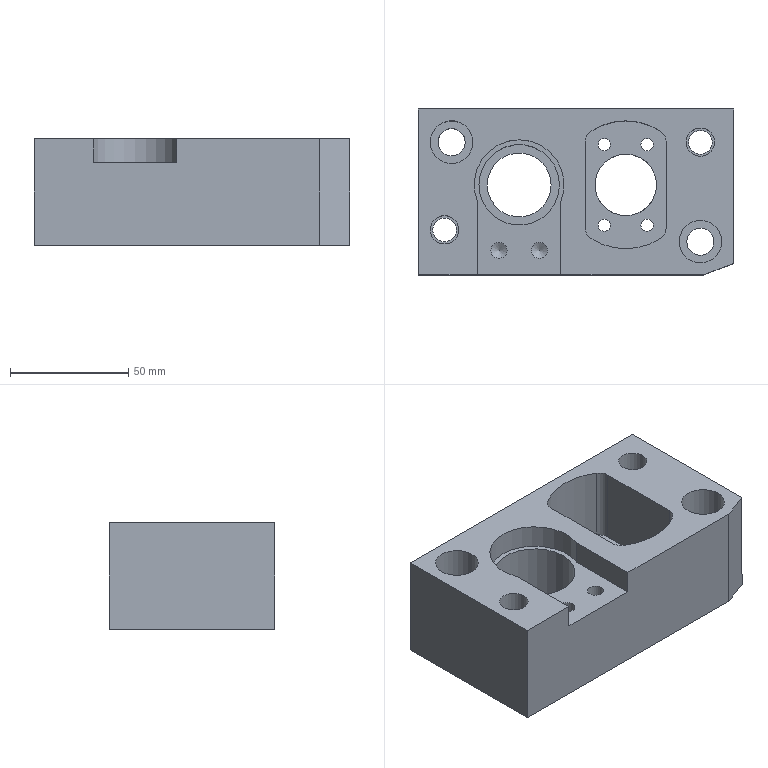Part | NX | features 26 2 | 1 solid | 44 faces | box 133 x 70 x 45 mm | volume 280682 mm3 | cylinder 24 | plane 18 | cone 2 | commonest cylinder face diameters 5.2 x4 10 x4 6.8 x2 10.001 x2 11.5 x2 12 x2
STEP:
#1=CARTESIAN_POINT('',(3287.,18.439,-68.));
#2=VERTEX_POINT('',#1);
#3=CARTESIAN_POINT('',(3287.,-18.439,-68.));
#4=VERTEX_POINT('',#3);
#5=CARTESIAN_POINT('',(3287.,211.,-68.));
#6=DIRECTION('',(0.,-1.,0.));
#7=VECTOR('',#6,1000.);
#8=LINE('',#5,#7);
#9=EDGE_CURVE('',#2,#4,#8,.T.);
#10=ORIENTED_EDGE('',*,*,#9,.F.);
#11=CARTESIAN_POINT('',(3289.273,22.63,-68.));
#12=VERTEX_POINT('',#11);
#13=CARTESIAN_POINT('',(3292.,18.439,-68.));
#14=DIRECTION('',(0.,0.,1.));
#15=DIRECTION('',(1.,0.,0.));
#16=AXIS2_PLACEMENT_3D('',#13,#14,#15);
#17=CIRCLE('',#16,5.);
#18=EDGE_CURVE('',#12,#2,#17,.T.);
#19=ORIENTED_EDGE('',*,*,#18,.F.);
#20=CARTESIAN_POINT('',(3318.727,22.63,-68.));
#21=VERTEX_POINT('',#20);
#22=CARTESIAN_POINT('',(3304.,0.,-68.));
#23=DIRECTION('',(0.,0.,1.));
#24=DIRECTION('',(1.,0.,0.));
#25=AXIS2_PLACEMENT_3D('',#22,#23,#24);
#26=CIRCLE('',#25,27.);
#27=EDGE_CURVE('',#21,#12,#26,.T.);
#28=ORIENTED_EDGE('',*,*,#27,.F.);
#29=CARTESIAN_POINT('',(3321.,18.439,-68.));
#30=VERTEX_POINT('',#29);
#31=CARTESIAN_POINT('',(3316.,18.439,-68.));
#32=DIRECTION('',(0.,0.,1.));
#33=DIRECTION('',(1.,0.,0.));
#34=AXIS2_PLACEMENT_3D('',#31,#32,#33);
#35=CIRCLE('',#34,5.);
#36=EDGE_CURVE('',#30,#21,#35,.T.);
#37=ORIENTED_EDGE('',*,*,#36,.F.);
#38=CARTESIAN_POINT('',(3321.,-18.439,-68.));
#39=VERTEX_POINT('',#38);
#40=CARTESIAN_POINT('',(3321.,211.,-68.));
#41=DIRECTION('',(0.,1.,0.));
#42=VECTOR('',#41,1000.);
#43=LINE('',#40,#42);
#44=EDGE_CURVE('',#39,#30,#43,.T.);
#45=ORIENTED_EDGE('',*,*,#44,.F.);
#46=CARTESIAN_POINT('',(3318.727,-22.63,-68.));
#47=VERTEX_POINT('',#46);
#48=CARTESIAN_POINT('',(3316.,-18.439,-68.));
#49=DIRECTION('',(0.,0.,1.));
#50=DIRECTION('',(1.,0.,0.));
#51=AXIS2_PLACEMENT_3D('',#48,#49,#50);
#52=CIRCLE('',#51,5.);
#53=EDGE_CURVE('',#47,#39,#52,.T.);
#54=ORIENTED_EDGE('',*,*,#53,.F.);
#55=CARTESIAN_POINT('',(3289.273,-22.63,-68.));
#56=VERTEX_POINT('',#55);
#57=CARTESIAN_POINT('',(3304.,0.,-68.));
#58=DIRECTION('',(0.,0.,1.));
#59=DIRECTION('',(1.,0.,0.));
#60=AXIS2_PLACEMENT_3D('',#57,#58,#59);
#61=CIRCLE('',#60,27.);
#62=EDGE_CURVE('',#56,#47,#61,.T.);
#63=ORIENTED_EDGE('',*,*,#62,.F.);
#64=CARTESIAN_POINT('',(3292.,-18.439,-68.));
#65=DIRECTION('',(0.,0.,1.));
#66=DIRECTION('',(1.,0.,0.));
#67=AXIS2_PLACEMENT_3D('',#64,#65,#66);
#68=CIRCLE('',#67,5.);
#69=EDGE_CURVE('',#4,#56,#68,.T.);
#70=ORIENTED_EDGE('',*,*,#69,.F.);
#71=EDGE_LOOP('',(#10,#19,#28,#37,#45,#54,#63,#70));
#72=FACE_BOUND('',#71,.T.);
#73=CARTESIAN_POINT('',(3326.5,-24.,-68.));
#74=VERTEX_POINT('',#73);
#75=CARTESIAN_POINT('',(3335.5,-24.,-68.));
#76=DIRECTION('',(0.,0.,1.));
#77=DIRECTION('',(-1.,0.,0.));
#78=AXIS2_PLACEMENT_3D('',#75,#76,#77);
#79=CIRCLE('',#78,9.);
#80=EDGE_CURVE('',#74,#74,#79,.T.);
#81=ORIENTED_EDGE('',*,*,#80,.F.);
#82=EDGE_LOOP('',(#81));
#83=FACE_BOUND('',#82,.T.);
#84=CARTESIAN_POINT('',(3221.5,18.,-68.));
#85=VERTEX_POINT('',#84);
#86=CARTESIAN_POINT('',(3230.5,18.,-68.));
#87=DIRECTION('',(0.,0.,1.));
#88=DIRECTION('',(-1.,0.,0.));
#89=AXIS2_PLACEMENT_3D('',#86,#87,#88);
#90=CIRCLE('',#89,9.);
#91=EDGE_CURVE('',#85,#85,#90,.T.);
#92=ORIENTED_EDGE('',*,*,#91,.F.);
#93=EDGE_LOOP('',(#92));
#94=FACE_BOUND('',#93,.T.);
#95=CARTESIAN_POINT('',(3233.5,-19.,-68.));
#96=VERTEX_POINT('',#95);
#97=CARTESIAN_POINT('',(3227.5,-19.,-68.));
#98=DIRECTION('',(0.,0.,-1.));
#99=DIRECTION('',(1.,0.,0.));
#100=AXIS2_PLACEMENT_3D('',#97,#98,#99);
#101=CIRCLE('',#100,6.);
#102=EDGE_CURVE('',#96,#96,#101,.T.);
#103=ORIENTED_EDGE('',*,*,#102,.T.);
#104=EDGE_LOOP('',(#103));
#105=FACE_BOUND('',#104,.T.);
#106=CARTESIAN_POINT('',(3341.5,18.,-68.));
#107=VERTEX_POINT('',#106);
#108=CARTESIAN_POINT('',(3335.5,18.,-68.));
#109=DIRECTION('',(0.,0.,-1.));
#110=DIRECTION('',(1.,0.,0.));
#111=AXIS2_PLACEMENT_3D('',#108,#109,#110);
#112=CIRCLE('',#111,6.);
#113=EDGE_CURVE('',#107,#107,#112,.T.);
#114=ORIENTED_EDGE('',*,*,#113,.T.);
#115=EDGE_LOOP('',(#114));
#116=FACE_BOUND('',#115,.T.);
#117=CARTESIAN_POINT('',(3349.5,-33.209,-68.));
#118=VERTEX_POINT('',#117);
#119=CARTESIAN_POINT('',(3336.859,-38.,-68.));
#120=VERTEX_POINT('',#119);
#121=CARTESIAN_POINT('',(4367.889,352.74,-68.));
#122=DIRECTION('',(-0.9351,-0.3544,0.));
#123=VECTOR('',#122,1000.);
#124=LINE('',#121,#123);
#125=EDGE_CURVE('',#118,#120,#124,.T.);
#126=ORIENTED_EDGE('',*,*,#125,.F.);
#127=CARTESIAN_POINT('',(3349.5,32.,-68.));
#128=VERTEX_POINT('',#127);
#129=CARTESIAN_POINT('',(3349.5,0.,-68.));
#130=DIRECTION('',(0.,1.,0.));
#131=VECTOR('',#130,1000.);
#132=LINE('',#129,#131);
#133=EDGE_CURVE('',#118,#128,#132,.T.);
#134=ORIENTED_EDGE('',*,*,#133,.T.);
#135=CARTESIAN_POINT('',(3216.5,32.,-68.));
#136=VERTEX_POINT('',#135);
#137=CARTESIAN_POINT('',(3259.,32.,-68.));
#138=DIRECTION('',(-1.,0.,0.));
#139=VECTOR('',#138,1000.);
#140=LINE('',#137,#139);
#141=EDGE_CURVE('',#128,#136,#140,.T.);
#142=ORIENTED_EDGE('',*,*,#141,.T.);
#143=CARTESIAN_POINT('',(3216.5,-38.,-68.));
#144=VERTEX_POINT('',#143);
#145=CARTESIAN_POINT('',(3216.5,0.,-68.));
#146=DIRECTION('',(0.,-1.,0.));
#147=VECTOR('',#146,1000.);
#148=LINE('',#145,#147);
#149=EDGE_CURVE('',#136,#144,#148,.T.);
#150=ORIENTED_EDGE('',*,*,#149,.T.);
#151=CARTESIAN_POINT('',(3241.4,-38.,-68.));
#152=VERTEX_POINT('',#151);
#153=CARTESIAN_POINT('',(3259.,-38.,-68.));
#154=DIRECTION('',(1.,0.,0.));
#155=VECTOR('',#154,1000.);
#156=LINE('',#153,#155);
#157=EDGE_CURVE('',#144,#152,#156,.T.);
#158=ORIENTED_EDGE('',*,*,#157,.T.);
#159=CARTESIAN_POINT('',(3241.4,-7.158,-68.));
#160=VERTEX_POINT('',#159);
#161=CARTESIAN_POINT('',(3241.4,206.,-68.));
#162=DIRECTION('',(0.,-1.,0.));
#163=VECTOR('',#162,1000.);
#164=LINE('',#161,#163);
#165=EDGE_CURVE('',#160,#152,#164,.T.);
#166=ORIENTED_EDGE('',*,*,#165,.F.);
#167=CARTESIAN_POINT('',(3276.6,-7.158,-68.));
#168=VERTEX_POINT('',#167);
#169=CARTESIAN_POINT('',(3259.,0.,-68.));
#170=DIRECTION('',(0.,0.,1.));
#171=DIRECTION('',(-1.,0.,0.));
#172=AXIS2_PLACEMENT_3D('',#169,#170,#171);
#173=CIRCLE('',#172,19.);
#174=EDGE_CURVE('',#168,#160,#173,.T.);
#175=ORIENTED_EDGE('',*,*,#174,.F.);
#176=CARTESIAN_POINT('',(3276.6,-38.,-68.));
#177=VERTEX_POINT('',#176);
#178=CARTESIAN_POINT('',(3276.6,206.,-68.));
#179=DIRECTION('',(0.,1.,0.));
#180=VECTOR('',#179,1000.);
#181=LINE('',#178,#180);
#182=EDGE_CURVE('',#177,#168,#181,.T.);
#183=ORIENTED_EDGE('',*,*,#182,.F.);
#184=CARTESIAN_POINT('',(3259.,-38.,-68.));
#185=DIRECTION('',(1.,0.,0.));
#186=VECTOR('',#185,1000.);
#187=LINE('',#184,#186);
#188=EDGE_CURVE('',#177,#120,#187,.T.);
#189=ORIENTED_EDGE('',*,*,#188,.T.);
#190=EDGE_LOOP('',(#126,#134,#142,#150,#158,#166,#175,#183,#189));
#191=FACE_BOUND('',#190,.T.);
#192=CARTESIAN_POINT('',(4423.5,206.,-68.));
#193=DIRECTION('',(0.,0.,-1.));
#194=DIRECTION('',(1.,0.,0.));
#195=AXIS2_PLACEMENT_3D('',#192,#193,#194);
#196=PLANE('',#195);
#197=ADVANCED_FACE('',(#72,#83,#94,#105,#116,#191),#196,.F.);
#198=ORIENTED_EDGE('',*,*,#133,.F.);
#199=CARTESIAN_POINT('',(3349.5,-33.209,-113.));
#200=VERTEX_POINT('',#199);
#201=CARTESIAN_POINT('',(3349.5,-33.209,-123.5));
#202=DIRECTION('',(0.,0.,-1.));
#203=VECTOR('',#202,1000.);
#204=LINE('',#201,#203);
#205=EDGE_CURVE('',#118,#200,#204,.T.);
#206=ORIENTED_EDGE('',*,*,#205,.T.);
#207=CARTESIAN_POINT('',(3349.5,32.,-113.));
#208=VERTEX_POINT('',#207);
#209=CARTESIAN_POINT('',(3349.5,0.,-113.));
#210=DIRECTION('',(0.,-1.,0.));
#211=VECTOR('',#210,1000.);
#212=LINE('',#209,#211);
#213=EDGE_CURVE('',#208,#200,#212,.T.);
#214=ORIENTED_EDGE('',*,*,#213,.F.);
#215=CARTESIAN_POINT('',(3349.5,32.,-123.5));
#216=DIRECTION('',(0.,0.,1.));
#217=VECTOR('',#216,1000.);
#218=LINE('',#215,#217);
#219=EDGE_CURVE('',#208,#128,#218,.T.);
#220=ORIENTED_EDGE('',*,*,#219,.T.);
#221=EDGE_LOOP('',(#198,#206,#214,#220));
#222=FACE_BOUND('',#221,.T.);
#223=CARTESIAN_POINT('',(3349.5,0.,-123.5));
#224=DIRECTION('',(1.,0.,0.));
#225=DIRECTION('',(0.,0.,1.));
#226=AXIS2_PLACEMENT_3D('',#223,#224,#225);
#227=PLANE('',#226);
#228=ADVANCED_FACE('',(#222),#227,.T.);
#229=CARTESIAN_POINT('',(3336.859,-38.,-113.));
#230=VERTEX_POINT('',#229);
#231=CARTESIAN_POINT('',(3216.5,-38.,-113.));
#232=VERTEX_POINT('',#231);
#233=CARTESIAN_POINT('',(3259.,-38.,-113.));
#234=DIRECTION('',(-1.,0.,0.));
#235=VECTOR('',#234,1000.);
#236=LINE('',#233,#235);
#237=EDGE_CURVE('',#230,#232,#236,.T.);
#238=ORIENTED_EDGE('',*,*,#237,.F.);
#239=CARTESIAN_POINT('',(3336.859,-38.,-123.5));
#240=DIRECTION('',(0.,0.,1.));
#241=VECTOR('',#240,1000.);
#242=LINE('',#239,#241);
#243=EDGE_CURVE('',#230,#120,#242,.T.);
#244=ORIENTED_EDGE('',*,*,#243,.T.);
#245=ORIENTED_EDGE('',*,*,#188,.F.);
#246=CARTESIAN_POINT('',(3276.6,-38.,-78.));
#247=VERTEX_POINT('',#246);
#248=CARTESIAN_POINT('',(3276.6,-38.,-123.5));
#249=DIRECTION('',(0.,0.,-1.));
#250=VECTOR('',#249,1000.);
#251=LINE('',#248,#250);
#252=EDGE_CURVE('',#177,#247,#251,.T.);
#253=ORIENTED_EDGE('',*,*,#252,.T.);
#254=CARTESIAN_POINT('',(3241.4,-38.,-78.));
#255=VERTEX_POINT('',#254);
#256=CARTESIAN_POINT('',(3259.,-38.,-78.));
#257=DIRECTION('',(-1.,0.,0.));
#258=VECTOR('',#257,1000.);
#259=LINE('',#256,#258);
#260=EDGE_CURVE('',#247,#255,#259,.T.);
#261=ORIENTED_EDGE('',*,*,#260,.T.);
#262=CARTESIAN_POINT('',(3241.4,-38.,-58.));
#263=DIRECTION('',(0.,0.,-1.));
#264=VECTOR('',#263,1000.);
#265=LINE('',#262,#264);
#266=EDGE_CURVE('',#152,#255,#265,.T.);
#267=ORIENTED_EDGE('',*,*,#266,.F.);
#268=ORIENTED_EDGE('',*,*,#157,.F.);
#269=CARTESIAN_POINT('',(3216.5,-38.,-123.5));
#270=DIRECTION('',(0.,0.,1.));
#271=VECTOR('',#270,1000.);
#272=LINE('',#269,#271);
#273=EDGE_CURVE('',#232,#144,#272,.T.);
#274=ORIENTED_EDGE('',*,*,#273,.F.);
#275=EDGE_LOOP('',(#238,#244,#245,#253,#261,#267,#268,#274));
#276=FACE_BOUND('',#275,.T.);
#277=CARTESIAN_POINT('',(3259.,-38.,-123.5));
#278=DIRECTION('',(0.,-1.,0.));
#279=DIRECTION('',(0.,0.,-1.));
#280=AXIS2_PLACEMENT_3D('',#277,#278,#279);
#281=PLANE('',#280);
#282=ADVANCED_FACE('',(#276),#281,.T.);
#283=CARTESIAN_POINT('',(3292.4,17.,-113.));
#284=VERTEX_POINT('',#283);
#285=CARTESIAN_POINT('',(3295.,17.,-113.));
#286=DIRECTION('',(0.,0.,-1.));
#287=DIRECTION('',(-1.,0.,0.));
#288=AXIS2_PLACEMENT_3D('',#285,#286,#287);
#289=CIRCLE('',#288,2.6);
#290=EDGE_CURVE('',#284,#284,#289,.T.);
#291=ORIENTED_EDGE('',*,*,#290,.F.);
#292=EDGE_LOOP('',(#291));
#293=FACE_BOUND('',#292,.T.);
#294=CARTESIAN_POINT('',(3292.4,-17.,-113.));
#295=VERTEX_POINT('',#294);
#296=CARTESIAN_POINT('',(3295.,-17.,-113.));
#297=DIRECTION('',(0.,0.,-1.));
#298=DIRECTION('',(-1.,0.,0.));
#299=AXIS2_PLACEMENT_3D('',#296,#297,#298);
#300=CIRCLE('',#299,2.6);
#301=EDGE_CURVE('',#295,#295,#300,.T.);
#302=ORIENTED_EDGE('',*,*,#301,.F.);
#303=EDGE_LOOP('',(#302));
#304=FACE_BOUND('',#303,.T.);
#305=CARTESIAN_POINT('',(3310.4,17.,-113.));
#306=VERTEX_POINT('',#305);
#307=CARTESIAN_POINT('',(3313.,17.,-113.));
#308=DIRECTION('',(0.,0.,-1.));
#309=DIRECTION('',(-1.,0.,0.));
#310=AXIS2_PLACEMENT_3D('',#307,#308,#309);
#311=CIRCLE('',#310,2.6);
#312=EDGE_CURVE('',#306,#306,#311,.T.);
#313=ORIENTED_EDGE('',*,*,#312,.F.);
#314=EDGE_LOOP('',(#313));
#315=FACE_BOUND('',#314,.T.);
#316=CARTESIAN_POINT('',(3310.4,-17.,-113.));
#317=VERTEX_POINT('',#316);
#318=CARTESIAN_POINT('',(3313.,-17.,-113.));
#319=DIRECTION('',(0.,0.,-1.));
#320=DIRECTION('',(-1.,0.,0.));
#321=AXIS2_PLACEMENT_3D('',#318,#319,#320);
#322=CIRCLE('',#321,2.6);
#323=EDGE_CURVE('',#317,#317,#322,.T.);
#324=ORIENTED_EDGE('',*,*,#323,.F.);
#325=EDGE_LOOP('',(#324));
#326=FACE_BOUND('',#325,.T.);
#327=CARTESIAN_POINT('',(3222.499,-19.,-113.));
#328=VERTEX_POINT('',#327);
#329=CARTESIAN_POINT('',(3227.5,-19.,-113.));
#330=DIRECTION('',(0.,0.,-1.));
#331=DIRECTION('',(-1.,0.,0.));
#332=AXIS2_PLACEMENT_3D('',#329,#330,#331);
#333=CIRCLE('',#332,5.);
#334=EDGE_CURVE('',#328,#328,#333,.T.);
#335=ORIENTED_EDGE('',*,*,#334,.F.);
#336=EDGE_LOOP('',(#335));
#337=FACE_BOUND('',#336,.T.);
#338=CARTESIAN_POINT('',(3224.75,18.,-113.));
#339=VERTEX_POINT('',#338);
#340=CARTESIAN_POINT('',(3230.5,18.,-113.));
#341=DIRECTION('',(0.,0.,-1.));
#342=DIRECTION('',(-1.,0.,0.));
#343=AXIS2_PLACEMENT_3D('',#340,#341,#342);
#344=CIRCLE('',#343,5.75);
#345=EDGE_CURVE('',#339,#339,#344,.T.);
#346=ORIENTED_EDGE('',*,*,#345,.F.);
#347=EDGE_LOOP('',(#346));
#348=FACE_BOUND('',#347,.T.);
#349=CARTESIAN_POINT('',(3245.5,0.,-113.));
#350=VERTEX_POINT('',#349);
#351=CARTESIAN_POINT('',(3259.,0.,-113.));
#352=DIRECTION('',(0.,0.,-1.));
#353=DIRECTION('',(-1.,0.,0.));
#354=AXIS2_PLACEMENT_3D('',#351,#352,#353);
#355=CIRCLE('',#354,13.5);
#356=EDGE_CURVE('',#350,#350,#355,.T.);
#357=ORIENTED_EDGE('',*,*,#356,.F.);
#358=EDGE_LOOP('',(#357));
#359=FACE_BOUND('',#358,.T.);
#360=CARTESIAN_POINT('',(3329.75,-24.,-113.));
#361=VERTEX_POINT('',#360);
#362=CARTESIAN_POINT('',(3335.5,-24.,-113.));
#363=DIRECTION('',(0.,0.,-1.));
#364=DIRECTION('',(-1.,0.,0.));
#365=AXIS2_PLACEMENT_3D('',#362,#363,#364);
#366=CIRCLE('',#365,5.75);
#367=EDGE_CURVE('',#361,#361,#366,.T.);
#368=ORIENTED_EDGE('',*,*,#367,.F.);
#369=EDGE_LOOP('',(#368));
#370=FACE_BOUND('',#369,.T.);
#371=CARTESIAN_POINT('',(3330.499,18.,-113.));
#372=VERTEX_POINT('',#371);
#373=CARTESIAN_POINT('',(3335.5,18.,-113.));
#374=DIRECTION('',(0.,0.,-1.));
#375=DIRECTION('',(-1.,0.,0.));
#376=AXIS2_PLACEMENT_3D('',#373,#374,#375);
#377=CIRCLE('',#376,5.);
#378=EDGE_CURVE('',#372,#372,#377,.T.);
#379=ORIENTED_EDGE('',*,*,#378,.F.);
#380=EDGE_LOOP('',(#379));
#381=FACE_BOUND('',#380,.T.);
#382=CARTESIAN_POINT('',(3317.,0.,-113.));
#383=VERTEX_POINT('',#382);
#384=CARTESIAN_POINT('',(3304.,0.,-113.));
#385=DIRECTION('',(0.,0.,1.));
#386=DIRECTION('',(1.,0.,0.));
#387=AXIS2_PLACEMENT_3D('',#384,#385,#386);
#388=CIRCLE('',#387,13.);
#389=EDGE_CURVE('',#383,#383,#388,.T.);
#390=ORIENTED_EDGE('',*,*,#389,.T.);
#391=EDGE_LOOP('',(#390));
#392=FACE_BOUND('',#391,.T.);
#393=ORIENTED_EDGE('',*,*,#213,.T.);
#394=CARTESIAN_POINT('',(4355.903,348.197,-113.));
#395=DIRECTION('',(-0.9351,-0.3544,0.));
#396=VECTOR('',#395,1000.);
#397=LINE('',#394,#396);
#398=EDGE_CURVE('',#200,#230,#397,.T.);
#399=ORIENTED_EDGE('',*,*,#398,.T.);
#400=ORIENTED_EDGE('',*,*,#237,.T.);
#401=CARTESIAN_POINT('',(3216.5,32.,-113.));
#402=VERTEX_POINT('',#401);
#403=CARTESIAN_POINT('',(3216.5,0.,-113.));
#404=DIRECTION('',(0.,1.,0.));
#405=VECTOR('',#404,1000.);
#406=LINE('',#403,#405);
#407=EDGE_CURVE('',#232,#402,#406,.T.);
#408=ORIENTED_EDGE('',*,*,#407,.T.);
#409=CARTESIAN_POINT('',(3259.,32.,-113.));
#410=DIRECTION('',(1.,0.,0.));
#411=VECTOR('',#410,1000.);
#412=LINE('',#409,#411);
#413=EDGE_CURVE('',#402,#208,#412,.T.);
#414=ORIENTED_EDGE('',*,*,#413,.T.);
#415=EDGE_LOOP('',(#393,#399,#400,#408,#414));
#416=FACE_BOUND('',#415,.T.);
#417=CARTESIAN_POINT('',(4489.,-3.,-113.));
#418=DIRECTION('',(0.,0.,-1.));
#419=DIRECTION('',(-1.,0.,0.));
#420=AXIS2_PLACEMENT_3D('',#417,#418,#419);
#421=PLANE('',#420);
#422=ADVANCED_FACE('',(#293,#304,#315,#326,#337,#348,#359,#370,#381,#392,#416),#421,.T.);
#423=CARTESIAN_POINT('',(3276.,0.,-108.));
#424=VERTEX_POINT('',#423);
#425=CARTESIAN_POINT('',(3259.,0.,-108.));
#426=DIRECTION('',(0.,0.,1.));
#427=DIRECTION('',(1.,0.,0.));
#428=AXIS2_PLACEMENT_3D('',#425,#426,#427);
#429=CIRCLE('',#428,17.);
#430=EDGE_CURVE('',#424,#424,#429,.T.);
#431=ORIENTED_EDGE('',*,*,#430,.F.);
#432=EDGE_LOOP('',(#431));
#433=FACE_BOUND('',#432,.T.);
#434=CARTESIAN_POINT('',(3276.,0.,-78.));
#435=VERTEX_POINT('',#434);
#436=CARTESIAN_POINT('',(3259.,0.,-78.));
#437=DIRECTION('',(0.,0.,-1.));
#438=DIRECTION('',(1.,0.,0.));
#439=AXIS2_PLACEMENT_3D('',#436,#437,#438);
#440=CIRCLE('',#439,17.);
#441=EDGE_CURVE('',#435,#435,#440,.T.);
#442=ORIENTED_EDGE('',*,*,#441,.F.);
#443=EDGE_LOOP('',(#442));
#444=FACE_BOUND('',#443,.T.);
#445=CARTESIAN_POINT('',(3259.,0.,512.));
#446=DIRECTION('',(0.,0.,-1.));
#447=DIRECTION('',(1.,0.,0.));
#448=AXIS2_PLACEMENT_3D('',#445,#446,#447);
#449=CYLINDRICAL_SURFACE('',#448,17.);
#450=ADVANCED_FACE('',(#433,#444),#449,.F.);
#451=ORIENTED_EDGE('',*,*,#273,.T.);
#452=ORIENTED_EDGE('',*,*,#149,.F.);
#453=CARTESIAN_POINT('',(3216.5,32.,-123.5));
#454=DIRECTION('',(0.,0.,1.));
#455=VECTOR('',#454,1000.);
#456=LINE('',#453,#455);
#457=EDGE_CURVE('',#402,#136,#456,.T.);
#458=ORIENTED_EDGE('',*,*,#457,.F.);
#459=ORIENTED_EDGE('',*,*,#407,.F.);
#460=EDGE_LOOP('',(#451,#452,#458,#459));
#461=FACE_BOUND('',#460,.T.);
#462=CARTESIAN_POINT('',(3216.5,0.,-123.5));
#463=DIRECTION('',(-1.,0.,0.));
#464=DIRECTION('',(0.,0.,-1.));
#465=AXIS2_PLACEMENT_3D('',#462,#463,#464);
#466=PLANE('',#465);
#467=ADVANCED_FACE('',(#461),#466,.T.);
#468=ORIENTED_EDGE('',*,*,#457,.T.);
#469=ORIENTED_EDGE('',*,*,#141,.F.);
#470=ORIENTED_EDGE('',*,*,#219,.F.);
#471=ORIENTED_EDGE('',*,*,#413,.F.);
#472=EDGE_LOOP('',(#468,#469,#470,#471));
#473=FACE_BOUND('',#472,.T.);
#474=CARTESIAN_POINT('',(3259.,32.,-123.5));
#475=DIRECTION('',(0.,1.,0.));
#476=DIRECTION('',(0.,0.,1.));
#477=AXIS2_PLACEMENT_3D('',#474,#475,#476);
#478=PLANE('',#477);
#479=ADVANCED_FACE('',(#473),#478,.T.);
#480=CARTESIAN_POINT('',(3222.499,-19.,-88.5));
#481=VERTEX_POINT('',#480);
#482=CARTESIAN_POINT('',(3227.5,-19.,-88.5));
#483=DIRECTION('',(0.,0.,1.));
#484=DIRECTION('',(-1.,0.,0.));
#485=AXIS2_PLACEMENT_3D('',#482,#483,#484);
#486=CIRCLE('',#485,5.);
#487=EDGE_CURVE('',#481,#481,#486,.T.);
#488=ORIENTED_EDGE('',*,*,#487,.T.);
#489=EDGE_LOOP('',(#488));
#490=FACE_BOUND('',#489,.T.);
#491=ORIENTED_EDGE('',*,*,#334,.T.);
#492=EDGE_LOOP('',(#491));
#493=FACE_BOUND('',#492,.T.);
#494=CARTESIAN_POINT('',(3227.5,-19.,541.5));
#495=DIRECTION('',(0.,0.,-1.));
#496=DIRECTION('',(1.,0.,0.));
#497=AXIS2_PLACEMENT_3D('',#494,#495,#496);
#498=CYLINDRICAL_SURFACE('',#497,5.);
#499=ADVANCED_FACE('',(#490,#493),#498,.F.);
#500=CARTESIAN_POINT('',(3330.499,18.,-88.5));
#501=VERTEX_POINT('',#500);
#502=CARTESIAN_POINT('',(3335.5,18.,-88.5));
#503=DIRECTION('',(0.,0.,1.));
#504=DIRECTION('',(-1.,0.,0.));
#505=AXIS2_PLACEMENT_3D('',#502,#503,#504);
#506=CIRCLE('',#505,5.);
#507=EDGE_CURVE('',#501,#501,#506,.T.);
#508=ORIENTED_EDGE('',*,*,#507,.T.);
#509=EDGE_LOOP('',(#508));
#510=FACE_BOUND('',#509,.T.);
#511=ORIENTED_EDGE('',*,*,#378,.T.);
#512=EDGE_LOOP('',(#511));
#513=FACE_BOUND('',#512,.T.);
#514=CARTESIAN_POINT('',(3335.5,18.,541.5));
#515=DIRECTION('',(0.,0.,-1.));
#516=DIRECTION('',(1.,0.,0.));
#517=AXIS2_PLACEMENT_3D('',#514,#515,#516);
#518=CYLINDRICAL_SURFACE('',#517,5.);
#519=ADVANCED_FACE('',(#510,#513),#518,.F.);
#520=CARTESIAN_POINT('',(3224.75,18.,-88.5));
#521=VERTEX_POINT('',#520);
#522=CARTESIAN_POINT('',(3230.5,18.,-88.5));
#523=DIRECTION('',(0.,0.,1.));
#524=DIRECTION('',(-1.,0.,0.));
#525=AXIS2_PLACEMENT_3D('',#522,#523,#524);
#526=CIRCLE('',#525,5.75);
#527=EDGE_CURVE('',#521,#521,#526,.T.);
#528=ORIENTED_EDGE('',*,*,#527,.T.);
#529=EDGE_LOOP('',(#528));
#530=FACE_BOUND('',#529,.T.);
#531=ORIENTED_EDGE('',*,*,#345,.T.);
#532=EDGE_LOOP('',(#531));
#533=FACE_BOUND('',#532,.T.);
#534=CARTESIAN_POINT('',(3230.5,18.,-66.5));
#535=DIRECTION('',(0.,0.,-1.));
#536=DIRECTION('',(-1.,0.,0.));
#537=AXIS2_PLACEMENT_3D('',#534,#535,#536);
#538=CYLINDRICAL_SURFACE('',#537,5.75);
#539=ADVANCED_FACE('',(#530,#533),#538,.F.);
#540=CARTESIAN_POINT('',(3329.75,-24.,-88.5));
#541=VERTEX_POINT('',#540);
#542=CARTESIAN_POINT('',(3335.5,-24.,-88.5));
#543=DIRECTION('',(0.,0.,1.));
#544=DIRECTION('',(-1.,0.,0.));
#545=AXIS2_PLACEMENT_3D('',#542,#543,#544);
#546=CIRCLE('',#545,5.75);
#547=EDGE_CURVE('',#541,#541,#546,.T.);
#548=ORIENTED_EDGE('',*,*,#547,.T.);
#549=EDGE_LOOP('',(#548));
#550=FACE_BOUND('',#549,.T.);
#551=ORIENTED_EDGE('',*,*,#367,.T.);
#552=EDGE_LOOP('',(#551));
#553=FACE_BOUND('',#552,.T.);
#554=CARTESIAN_POINT('',(3335.5,-24.,-66.5));
#555=DIRECTION('',(0.,0.,-1.));
#556=DIRECTION('',(-1.,0.,0.));
#557=AXIS2_PLACEMENT_3D('',#554,#555,#556);
#558=CYLINDRICAL_SURFACE('',#557,5.75);
#559=ADVANCED_FACE('',(#550,#553),#558,.F.);
#560=CARTESIAN_POINT('',(3272.5,0.,-108.));
#561=VERTEX_POINT('',#560);
#562=CARTESIAN_POINT('',(3259.,0.,-108.));
#563=DIRECTION('',(0.,0.,1.));
#564=DIRECTION('',(1.,0.,0.));
#565=AXIS2_PLACEMENT_3D('',#562,#563,#564);
#566=CIRCLE('',#565,13.5);
#567=EDGE_CURVE('',#561,#561,#566,.T.);
#568=ORIENTED_EDGE('',*,*,#567,.T.);
#569=EDGE_LOOP('',(#568));
#570=FACE_BOUND('',#569,.T.);
#571=ORIENTED_EDGE('',*,*,#356,.T.);
#572=EDGE_LOOP('',(#571));
#573=FACE_BOUND('',#572,.T.);
#574=CARTESIAN_POINT('',(3259.,0.,542.));
#575=DIRECTION('',(0.,0.,-1.));
#576=DIRECTION('',(1.,0.,0.));
#577=AXIS2_PLACEMENT_3D('',#574,#575,#576);
#578=CYLINDRICAL_SURFACE('',#577,13.5);
#579=ADVANCED_FACE('',(#570,#573),#578,.F.);
#580=CARTESIAN_POINT('',(3329.5,18.,-88.5));
#581=VERTEX_POINT('',#580);
#582=CARTESIAN_POINT('',(3335.5,18.,-88.5));
#583=DIRECTION('',(0.,0.,-1.));
#584=DIRECTION('',(-1.,0.,0.));
#585=AXIS2_PLACEMENT_3D('',#582,#583,#584);
#586=CIRCLE('',#585,6.);
#587=EDGE_CURVE('',#581,#581,#586,.T.);
#588=ORIENTED_EDGE('',*,*,#587,.T.);
#589=EDGE_LOOP('',(#588));
#590=FACE_BOUND('',#589,.T.);
#591=ORIENTED_EDGE('',*,*,#113,.F.);
#592=EDGE_LOOP('',(#591));
#593=FACE_BOUND('',#592,.T.);
#594=CARTESIAN_POINT('',(3335.5,18.,541.5));
#595=DIRECTION('',(0.,0.,-1.));
#596=DIRECTION('',(1.,0.,0.));
#597=AXIS2_PLACEMENT_3D('',#594,#595,#596);
#598=CYLINDRICAL_SURFACE('',#597,6.);
#599=ADVANCED_FACE('',(#590,#593),#598,.F.);
#600=CARTESIAN_POINT('',(3221.5,-19.,-88.5));
#601=VERTEX_POINT('',#600);
#602=CARTESIAN_POINT('',(3227.5,-19.,-88.5));
#603=DIRECTION('',(0.,0.,-1.));
#604=DIRECTION('',(-1.,0.,0.));
#605=AXIS2_PLACEMENT_3D('',#602,#603,#604);
#606=CIRCLE('',#605,6.);
#607=EDGE_CURVE('',#601,#601,#606,.T.);
#608=ORIENTED_EDGE('',*,*,#607,.T.);
#609=EDGE_LOOP('',(#608));
#610=FACE_BOUND('',#609,.T.);
#611=ORIENTED_EDGE('',*,*,#102,.F.);
#612=EDGE_LOOP('',(#611));
#613=FACE_BOUND('',#612,.T.);
#614=CARTESIAN_POINT('',(3227.5,-19.,541.5));
#615=DIRECTION('',(0.,0.,-1.));
#616=DIRECTION('',(1.,0.,0.));
#617=AXIS2_PLACEMENT_3D('',#614,#615,#616);
#618=CYLINDRICAL_SURFACE('',#617,6.);
#619=ADVANCED_FACE('',(#610,#613),#618,.F.);
#620=CARTESIAN_POINT('',(3221.5,18.,-88.5));
#621=VERTEX_POINT('',#620);
#622=CARTESIAN_POINT('',(3230.5,18.,-88.5));
#623=DIRECTION('',(0.,0.,1.));
#624=DIRECTION('',(-1.,0.,0.));
#625=AXIS2_PLACEMENT_3D('',#622,#623,#624);
#626=CIRCLE('',#625,9.);
#627=EDGE_CURVE('',#621,#621,#626,.T.);
#628=ORIENTED_EDGE('',*,*,#627,.F.);
#629=EDGE_LOOP('',(#628));
#630=FACE_BOUND('',#629,.T.);
#631=ORIENTED_EDGE('',*,*,#91,.T.);
#632=EDGE_LOOP('',(#631));
#633=FACE_BOUND('',#632,.T.);
#634=CARTESIAN_POINT('',(3230.5,18.,-68.5));
#635=DIRECTION('',(0.,0.,-1.));
#636=DIRECTION('',(-1.,0.,0.));
#637=AXIS2_PLACEMENT_3D('',#634,#635,#636);
#638=CYLINDRICAL_SURFACE('',#637,9.);
#639=ADVANCED_FACE('',(#630,#633),#638,.F.);
#640=CARTESIAN_POINT('',(3326.5,-24.,-88.5));
#641=VERTEX_POINT('',#640);
#642=CARTESIAN_POINT('',(3335.5,-24.,-88.5));
#643=DIRECTION('',(0.,0.,1.));
#644=DIRECTION('',(-1.,0.,0.));
#645=AXIS2_PLACEMENT_3D('',#642,#643,#644);
#646=CIRCLE('',#645,9.);
#647=EDGE_CURVE('',#641,#641,#646,.T.);
#648=ORIENTED_EDGE('',*,*,#647,.F.);
#649=EDGE_LOOP('',(#648));
#650=FACE_BOUND('',#649,.T.);
#651=ORIENTED_EDGE('',*,*,#80,.T.);
#652=EDGE_LOOP('',(#651));
#653=FACE_BOUND('',#652,.T.);
#654=CARTESIAN_POINT('',(3335.5,-24.,-68.5));
#655=DIRECTION('',(0.,0.,-1.));
#656=DIRECTION('',(-1.,0.,0.));
#657=AXIS2_PLACEMENT_3D('',#654,#655,#656);
#658=CYLINDRICAL_SURFACE('',#657,9.);
#659=ADVANCED_FACE('',(#650,#653),#658,.F.);
#660=ORIENTED_EDGE('',*,*,#647,.T.);
#661=EDGE_LOOP('',(#660));
#662=FACE_BOUND('',#661,.T.);
#663=ORIENTED_EDGE('',*,*,#547,.F.);
#664=EDGE_LOOP('',(#663));
#665=FACE_BOUND('',#664,.T.);
#666=CARTESIAN_POINT('',(3278.5,18.,-88.5));
#667=DIRECTION('',(0.,0.,-1.));
#668=DIRECTION('',(1.,0.,0.));
#669=AXIS2_PLACEMENT_3D('',#666,#667,#668);
#670=PLANE('',#669);
#671=ADVANCED_FACE('',(#662,#665),#670,.F.);
#672=ORIENTED_EDGE('',*,*,#587,.F.);
#673=EDGE_LOOP('',(#672));
#674=FACE_BOUND('',#673,.T.);
#675=ORIENTED_EDGE('',*,*,#507,.F.);
#676=EDGE_LOOP('',(#675));
#677=FACE_BOUND('',#676,.T.);
#678=CARTESIAN_POINT('',(3278.5,18.,-88.5));
#679=DIRECTION('',(0.,0.,-1.));
#680=DIRECTION('',(1.,0.,0.));
#681=AXIS2_PLACEMENT_3D('',#678,#679,#680);
#682=PLANE('',#681);
#683=ADVANCED_FACE('',(#674,#677),#682,.F.);
#684=ORIENTED_EDGE('',*,*,#607,.F.);
#685=EDGE_LOOP('',(#684));
#686=FACE_BOUND('',#685,.T.);
#687=ORIENTED_EDGE('',*,*,#487,.F.);
#688=EDGE_LOOP('',(#687));
#689=FACE_BOUND('',#688,.T.);
#690=CARTESIAN_POINT('',(3227.5,23.,-88.5));
#691=DIRECTION('',(0.,0.,-1.));
#692=DIRECTION('',(1.,0.,0.));
#693=AXIS2_PLACEMENT_3D('',#690,#691,#692);
#694=PLANE('',#693);
#695=ADVANCED_FACE('',(#686,#689),#694,.F.);
#696=ORIENTED_EDGE('',*,*,#430,.T.);
#697=EDGE_LOOP('',(#696));
#698=FACE_BOUND('',#697,.T.);
#699=ORIENTED_EDGE('',*,*,#567,.F.);
#700=EDGE_LOOP('',(#699));
#701=FACE_BOUND('',#700,.T.);
#702=CARTESIAN_POINT('',(3259.,0.,-108.));
#703=DIRECTION('',(0.,0.,1.));
#704=DIRECTION('',(-1.,0.,0.));
#705=AXIS2_PLACEMENT_3D('',#702,#703,#704);
#706=PLANE('',#705);
#707=ADVANCED_FACE('',(#698,#701),#706,.T.);
#708=ORIENTED_EDGE('',*,*,#627,.T.);
#709=EDGE_LOOP('',(#708));
#710=FACE_BOUND('',#709,.T.);
#711=ORIENTED_EDGE('',*,*,#527,.F.);
#712=EDGE_LOOP('',(#711));
#713=FACE_BOUND('',#712,.T.);
#714=CARTESIAN_POINT('',(3230.5,18.,-88.5));
#715=DIRECTION('',(0.,0.,-1.));
#716=DIRECTION('',(1.,0.,0.));
#717=AXIS2_PLACEMENT_3D('',#714,#715,#716);
#718=PLANE('',#717);
#719=ADVANCED_FACE('',(#710,#713),#718,.F.);
#720=CARTESIAN_POINT('',(3304.,13.,-100.));
#721=VERTEX_POINT('',#720);
#722=CARTESIAN_POINT('',(3304.,0.,-100.));
#723=DIRECTION('',(0.,0.,-1.));
#724=DIRECTION('',(0.,1.,0.));
#725=AXIS2_PLACEMENT_3D('',#722,#723,#724);
#726=CIRCLE('',#725,13.);
#727=EDGE_CURVE('',#721,#721,#726,.T.);
#728=ORIENTED_EDGE('',*,*,#727,.F.);
#729=EDGE_LOOP('',(#728));
#730=FACE_BOUND('',#729,.T.);
#731=ORIENTED_EDGE('',*,*,#389,.F.);
#732=EDGE_LOOP('',(#731));
#733=FACE_BOUND('',#732,.T.);
#734=CARTESIAN_POINT('',(3304.,0.,-95.5));
#735=DIRECTION('',(0.,0.,1.));
#736=DIRECTION('',(-1.,0.,0.));
#737=AXIS2_PLACEMENT_3D('',#734,#735,#736);
#738=CYLINDRICAL_SURFACE('',#737,13.);
#739=ADVANCED_FACE('',(#730,#733),#738,.F.);
#740=ORIENTED_EDGE('',*,*,#62,.T.);
#741=CARTESIAN_POINT('',(3318.727,-22.63,-100.));
#742=VERTEX_POINT('',#741);
#743=CARTESIAN_POINT('',(3318.727,-22.63,-95.5));
#744=DIRECTION('',(0.,0.,1.));
#745=VECTOR('',#744,1000.);
#746=LINE('',#743,#745);
#747=EDGE_CURVE('',#742,#47,#746,.T.);
#748=ORIENTED_EDGE('',*,*,#747,.F.);
#749=CARTESIAN_POINT('',(3289.273,-22.63,-100.));
#750=VERTEX_POINT('',#749);
#751=CARTESIAN_POINT('',(3304.,0.,-100.));
#752=DIRECTION('',(0.,0.,-1.));
#753=DIRECTION('',(0.,1.,0.));
#754=AXIS2_PLACEMENT_3D('',#751,#752,#753);
#755=CIRCLE('',#754,27.);
#756=EDGE_CURVE('',#742,#750,#755,.T.);
#757=ORIENTED_EDGE('',*,*,#756,.T.);
#758=CARTESIAN_POINT('',(3289.273,-22.63,-95.5));
#759=DIRECTION('',(0.,0.,-1.));
#760=VECTOR('',#759,1000.);
#761=LINE('',#758,#760);
#762=EDGE_CURVE('',#56,#750,#761,.T.);
#763=ORIENTED_EDGE('',*,*,#762,.F.);
#764=EDGE_LOOP('',(#740,#748,#757,#763));
#765=FACE_BOUND('',#764,.T.);
#766=CARTESIAN_POINT('',(3304.,0.,-95.5));
#767=DIRECTION('',(0.,0.,1.));
#768=DIRECTION('',(-1.,0.,0.));
#769=AXIS2_PLACEMENT_3D('',#766,#767,#768);
#770=CYLINDRICAL_SURFACE('',#769,27.);
#771=ADVANCED_FACE('',(#765),#770,.F.);
#772=CARTESIAN_POINT('',(3321.,18.439,-100.));
#773=VERTEX_POINT('',#772);
#774=CARTESIAN_POINT('',(3321.,-18.439,-100.));
#775=VERTEX_POINT('',#774);
#776=CARTESIAN_POINT('',(3321.,0.,-100.));
#777=DIRECTION('',(0.,-1.,0.));
#778=VECTOR('',#777,1000.);
#779=LINE('',#776,#778);
#780=EDGE_CURVE('',#773,#775,#779,.T.);
#781=ORIENTED_EDGE('',*,*,#780,.T.);
#782=CARTESIAN_POINT('',(3321.,-18.439,-100.));
#783=DIRECTION('',(0.,0.,-1.));
#784=VECTOR('',#783,1000.);
#785=LINE('',#782,#784);
#786=EDGE_CURVE('',#39,#775,#785,.T.);
#787=ORIENTED_EDGE('',*,*,#786,.F.);
#788=ORIENTED_EDGE('',*,*,#44,.T.);
#789=CARTESIAN_POINT('',(3321.,18.439,-68.5));
#790=DIRECTION('',(0.,0.,1.));
#791=VECTOR('',#790,1000.);
#792=LINE('',#789,#791);
#793=EDGE_CURVE('',#773,#30,#792,.T.);
#794=ORIENTED_EDGE('',*,*,#793,.F.);
#795=EDGE_LOOP('',(#781,#787,#788,#794));
#796=FACE_BOUND('',#795,.T.);
#797=CARTESIAN_POINT('',(3321.,0.,-95.5));
#798=DIRECTION('',(1.,0.,0.));
#799=DIRECTION('',(0.,-1.,0.));
#800=AXIS2_PLACEMENT_3D('',#797,#798,#799);
#801=PLANE('',#800);
#802=ADVANCED_FACE('',(#796),#801,.F.);
#803=ORIENTED_EDGE('',*,*,#27,.T.);
#804=CARTESIAN_POINT('',(3289.273,22.63,-100.));
#805=VERTEX_POINT('',#804);
#806=CARTESIAN_POINT('',(3289.273,22.63,-95.5));
#807=DIRECTION('',(0.,0.,1.));
#808=VECTOR('',#807,1000.);
#809=LINE('',#806,#808);
#810=EDGE_CURVE('',#805,#12,#809,.T.);
#811=ORIENTED_EDGE('',*,*,#810,.F.);
#812=CARTESIAN_POINT('',(3318.727,22.63,-100.));
#813=VERTEX_POINT('',#812);
#814=CARTESIAN_POINT('',(3304.,0.,-100.));
#815=DIRECTION('',(0.,0.,-1.));
#816=DIRECTION('',(0.,1.,0.));
#817=AXIS2_PLACEMENT_3D('',#814,#815,#816);
#818=CIRCLE('',#817,27.);
#819=EDGE_CURVE('',#805,#813,#818,.T.);
#820=ORIENTED_EDGE('',*,*,#819,.T.);
#821=CARTESIAN_POINT('',(3318.727,22.63,-95.5));
#822=DIRECTION('',(0.,0.,-1.));
#823=VECTOR('',#822,1000.);
#824=LINE('',#821,#823);
#825=EDGE_CURVE('',#21,#813,#824,.T.);
#826=ORIENTED_EDGE('',*,*,#825,.F.);
#827=EDGE_LOOP('',(#803,#811,#820,#826));
#828=FACE_BOUND('',#827,.T.);
#829=CARTESIAN_POINT('',(3304.,0.,-95.5));
#830=DIRECTION('',(0.,0.,1.));
#831=DIRECTION('',(-1.,0.,0.));
#832=AXIS2_PLACEMENT_3D('',#829,#830,#831);
#833=CYLINDRICAL_SURFACE('',#832,27.);
#834=ADVANCED_FACE('',(#828),#833,.F.);
#835=ORIENTED_EDGE('',*,*,#9,.T.);
#836=CARTESIAN_POINT('',(3287.,-18.439,-100.));
#837=VERTEX_POINT('',#836);
#838=CARTESIAN_POINT('',(3287.,-18.439,-68.5));
#839=DIRECTION('',(0.,0.,1.));
#840=VECTOR('',#839,1000.);
#841=LINE('',#838,#840);
#842=EDGE_CURVE('',#837,#4,#841,.T.);
#843=ORIENTED_EDGE('',*,*,#842,.F.);
#844=CARTESIAN_POINT('',(3287.,18.439,-100.));
#845=VERTEX_POINT('',#844);
#846=CARTESIAN_POINT('',(3287.,0.,-100.));
#847=DIRECTION('',(0.,1.,0.));
#848=VECTOR('',#847,1000.);
#849=LINE('',#846,#848);
#850=EDGE_CURVE('',#837,#845,#849,.T.);
#851=ORIENTED_EDGE('',*,*,#850,.T.);
#852=CARTESIAN_POINT('',(3287.,18.439,-100.));
#853=DIRECTION('',(0.,0.,-1.));
#854=VECTOR('',#853,1000.);
#855=LINE('',#852,#854);
#856=EDGE_CURVE('',#2,#845,#855,.T.);
#857=ORIENTED_EDGE('',*,*,#856,.F.);
#858=EDGE_LOOP('',(#835,#843,#851,#857));
#859=FACE_BOUND('',#858,.T.);
#860=CARTESIAN_POINT('',(3287.,0.,-95.5));
#861=DIRECTION('',(-1.,0.,0.));
#862=DIRECTION('',(0.,1.,0.));
#863=AXIS2_PLACEMENT_3D('',#860,#861,#862);
#864=PLANE('',#863);
#865=ADVANCED_FACE('',(#859),#864,.F.);
#866=CARTESIAN_POINT('',(3297.6,17.,-100.));
#867=VERTEX_POINT('',#866);
#868=CARTESIAN_POINT('',(3295.,17.,-100.));
#869=DIRECTION('',(0.,0.,-1.));
#870=DIRECTION('',(1.,0.,0.));
#871=AXIS2_PLACEMENT_3D('',#868,#869,#870);
#872=CIRCLE('',#871,2.6);
#873=EDGE_CURVE('',#867,#867,#872,.T.);
#874=ORIENTED_EDGE('',*,*,#873,.T.);
#875=EDGE_LOOP('',(#874));
#876=FACE_BOUND('',#875,.T.);
#877=CARTESIAN_POINT('',(3297.6,-17.,-100.));
#878=VERTEX_POINT('',#877);
#879=CARTESIAN_POINT('',(3295.,-17.,-100.));
#880=DIRECTION('',(0.,0.,-1.));
#881=DIRECTION('',(1.,0.,0.));
#882=AXIS2_PLACEMENT_3D('',#879,#880,#881);
#883=CIRCLE('',#882,2.6);
#884=EDGE_CURVE('',#878,#878,#883,.T.);
#885=ORIENTED_EDGE('',*,*,#884,.T.);
#886=EDGE_LOOP('',(#885));
#887=FACE_BOUND('',#886,.T.);
#888=CARTESIAN_POINT('',(3315.6,17.,-100.));
#889=VERTEX_POINT('',#888);
#890=CARTESIAN_POINT('',(3313.,17.,-100.));
#891=DIRECTION('',(0.,0.,-1.));
#892=DIRECTION('',(1.,0.,0.));
#893=AXIS2_PLACEMENT_3D('',#890,#891,#892);
#894=CIRCLE('',#893,2.6);
#895=EDGE_CURVE('',#889,#889,#894,.T.);
#896=ORIENTED_EDGE('',*,*,#895,.T.);
#897=EDGE_LOOP('',(#896));
#898=FACE_BOUND('',#897,.T.);
#899=CARTESIAN_POINT('',(3315.6,-17.,-100.));
#900=VERTEX_POINT('',#899);
#901=CARTESIAN_POINT('',(3313.,-17.,-100.));
#902=DIRECTION('',(0.,0.,-1.));
#903=DIRECTION('',(1.,0.,0.));
#904=AXIS2_PLACEMENT_3D('',#901,#902,#903);
#905=CIRCLE('',#904,2.6);
#906=EDGE_CURVE('',#900,#900,#905,.T.);
#907=ORIENTED_EDGE('',*,*,#906,.T.);
#908=EDGE_LOOP('',(#907));
#909=FACE_BOUND('',#908,.T.);
#910=ORIENTED_EDGE('',*,*,#727,.T.);
#911=EDGE_LOOP('',(#910));
#912=FACE_BOUND('',#911,.T.);
#913=ORIENTED_EDGE('',*,*,#819,.F.);
#914=CARTESIAN_POINT('',(3292.,18.439,-100.));
#915=DIRECTION('',(0.,0.,-1.));
#916=DIRECTION('',(0.,1.,0.));
#917=AXIS2_PLACEMENT_3D('',#914,#915,#916);
#918=CIRCLE('',#917,5.);
#919=EDGE_CURVE('',#845,#805,#918,.T.);
#920=ORIENTED_EDGE('',*,*,#919,.F.);
#921=ORIENTED_EDGE('',*,*,#850,.F.);
#922=CARTESIAN_POINT('',(3292.,-18.439,-100.));
#923=DIRECTION('',(0.,0.,-1.));
#924=DIRECTION('',(0.,1.,0.));
#925=AXIS2_PLACEMENT_3D('',#922,#923,#924);
#926=CIRCLE('',#925,5.);
#927=EDGE_CURVE('',#750,#837,#926,.T.);
#928=ORIENTED_EDGE('',*,*,#927,.F.);
#929=ORIENTED_EDGE('',*,*,#756,.F.);
#930=CARTESIAN_POINT('',(3316.,-18.439,-100.));
#931=DIRECTION('',(0.,0.,-1.));
#932=DIRECTION('',(0.,1.,0.));
#933=AXIS2_PLACEMENT_3D('',#930,#931,#932);
#934=CIRCLE('',#933,5.);
#935=EDGE_CURVE('',#775,#742,#934,.T.);
#936=ORIENTED_EDGE('',*,*,#935,.F.);
#937=ORIENTED_EDGE('',*,*,#780,.F.);
#938=CARTESIAN_POINT('',(3316.,18.439,-100.));
#939=DIRECTION('',(0.,0.,-1.));
#940=DIRECTION('',(0.,1.,0.));
#941=AXIS2_PLACEMENT_3D('',#938,#939,#940);
#942=CIRCLE('',#941,5.);
#943=EDGE_CURVE('',#813,#773,#942,.T.);
#944=ORIENTED_EDGE('',*,*,#943,.F.);
#945=EDGE_LOOP('',(#913,#920,#921,#928,#929,#936,#937,#944));
#946=FACE_BOUND('',#945,.T.);
#947=CARTESIAN_POINT('',(3304.,0.,-100.));
#948=DIRECTION('',(0.,0.,-1.));
#949=DIRECTION('',(1.,0.,0.));
#950=AXIS2_PLACEMENT_3D('',#947,#948,#949);
#951=PLANE('',#950);
#952=ADVANCED_FACE('',(#876,#887,#898,#909,#912,#946),#951,.F.);
#953=ORIENTED_EDGE('',*,*,#36,.T.);
#954=ORIENTED_EDGE('',*,*,#825,.T.);
#955=ORIENTED_EDGE('',*,*,#943,.T.);
#956=ORIENTED_EDGE('',*,*,#793,.T.);
#957=EDGE_LOOP('',(#953,#954,#955,#956));
#958=FACE_BOUND('',#957,.T.);
#959=CARTESIAN_POINT('',(3316.,18.439,-95.5));
#960=DIRECTION('',(0.,0.,1.));
#961=DIRECTION('',(0.,1.,0.));
#962=AXIS2_PLACEMENT_3D('',#959,#960,#961);
#963=CYLINDRICAL_SURFACE('',#962,5.);
#964=ADVANCED_FACE('',(#958),#963,.F.);
#965=ORIENTED_EDGE('',*,*,#919,.T.);
#966=ORIENTED_EDGE('',*,*,#810,.T.);
#967=ORIENTED_EDGE('',*,*,#18,.T.);
#968=ORIENTED_EDGE('',*,*,#856,.T.);
#969=EDGE_LOOP('',(#965,#966,#967,#968));
#970=FACE_BOUND('',#969,.T.);
#971=CARTESIAN_POINT('',(3292.,18.439,-95.5));
#972=DIRECTION('',(0.,0.,1.));
#973=DIRECTION('',(0.,1.,0.));
#974=AXIS2_PLACEMENT_3D('',#971,#972,#973);
#975=CYLINDRICAL_SURFACE('',#974,5.);
#976=ADVANCED_FACE('',(#970),#975,.F.);
#977=ORIENTED_EDGE('',*,*,#69,.T.);
#978=ORIENTED_EDGE('',*,*,#762,.T.);
#979=ORIENTED_EDGE('',*,*,#927,.T.);
#980=ORIENTED_EDGE('',*,*,#842,.T.);
#981=EDGE_LOOP('',(#977,#978,#979,#980));
#982=FACE_BOUND('',#981,.T.);
#983=CARTESIAN_POINT('',(3292.,-18.439,-95.5));
#984=DIRECTION('',(0.,0.,1.));
#985=DIRECTION('',(0.,1.,0.));
#986=AXIS2_PLACEMENT_3D('',#983,#984,#985);
#987=CYLINDRICAL_SURFACE('',#986,5.);
#988=ADVANCED_FACE('',(#982),#987,.F.);
#989=ORIENTED_EDGE('',*,*,#935,.T.);
#990=ORIENTED_EDGE('',*,*,#747,.T.);
#991=ORIENTED_EDGE('',*,*,#53,.T.);
#992=ORIENTED_EDGE('',*,*,#786,.T.);
#993=EDGE_LOOP('',(#989,#990,#991,#992));
#994=FACE_BOUND('',#993,.T.);
#995=CARTESIAN_POINT('',(3316.,-18.439,-95.5));
#996=DIRECTION('',(0.,0.,1.));
#997=DIRECTION('',(0.,1.,0.));
#998=AXIS2_PLACEMENT_3D('',#995,#996,#997);
#999=CYLINDRICAL_SURFACE('',#998,5.);
#1000=ADVANCED_FACE('',(#994),#999,.F.);
#1001=ORIENTED_EDGE('',*,*,#174,.T.);
#1002=CARTESIAN_POINT('',(3241.4,-7.158,-78.));
#1003=VERTEX_POINT('',#1002);
#1004=CARTESIAN_POINT('',(3241.4,-7.158,-78.));
#1005=DIRECTION('',(0.,0.,-1.));
#1006=VECTOR('',#1005,1000.);
#1007=LINE('',#1004,#1006);
#1008=EDGE_CURVE('',#160,#1003,#1007,.T.);
#1009=ORIENTED_EDGE('',*,*,#1008,.T.);
#1010=CARTESIAN_POINT('',(3276.6,-7.158,-78.));
#1011=VERTEX_POINT('',#1010);
#1012=CARTESIAN_POINT('',(3259.,0.,-78.));
#1013=DIRECTION('',(0.,0.,-1.));
#1014=DIRECTION('',(1.,0.,0.));
#1015=AXIS2_PLACEMENT_3D('',#1012,#1013,#1014);
#1016=CIRCLE('',#1015,19.);
#1017=EDGE_CURVE('',#1003,#1011,#1016,.T.);
#1018=ORIENTED_EDGE('',*,*,#1017,.T.);
#1019=CARTESIAN_POINT('',(3276.6,-7.158,-78.));
#1020=DIRECTION('',(0.,0.,1.));
#1021=VECTOR('',#1020,1000.);
#1022=LINE('',#1019,#1021);
#1023=EDGE_CURVE('',#1011,#168,#1022,.T.);
#1024=ORIENTED_EDGE('',*,*,#1023,.T.);
#1025=EDGE_LOOP('',(#1001,#1009,#1018,#1024));
#1026=FACE_BOUND('',#1025,.T.);
#1027=CARTESIAN_POINT('',(3259.,0.,-58.));
#1028=DIRECTION('',(0.,0.,-1.));
#1029=DIRECTION('',(1.,0.,0.));
#1030=AXIS2_PLACEMENT_3D('',#1027,#1028,#1029);
#1031=CYLINDRICAL_SURFACE('',#1030,19.);
#1032=ADVANCED_FACE('',(#1026),#1031,.F.);
#1033=CARTESIAN_POINT('',(3276.6,-13.,-78.));
#1034=DIRECTION('',(0.,-1.,0.));
#1035=VECTOR('',#1034,1000.);
#1036=LINE('',#1033,#1035);
#1037=EDGE_CURVE('',#1011,#247,#1036,.T.);
#1038=ORIENTED_EDGE('',*,*,#1037,.F.);
#1039=ORIENTED_EDGE('',*,*,#1017,.F.);
#1040=CARTESIAN_POINT('',(3241.4,-13.,-78.));
#1041=DIRECTION('',(0.,1.,0.));
#1042=VECTOR('',#1041,1000.);
#1043=LINE('',#1040,#1042);
#1044=EDGE_CURVE('',#255,#1003,#1043,.T.);
#1045=ORIENTED_EDGE('',*,*,#1044,.F.);
#1046=ORIENTED_EDGE('',*,*,#260,.F.);
#1047=EDGE_LOOP('',(#1038,#1039,#1045,#1046));
#1048=FACE_BOUND('',#1047,.T.);
#1049=CARTESIAN_POINT('',(3270.9,-27.7,-78.));
#1050=VERTEX_POINT('',#1049);
#1051=CARTESIAN_POINT('',(3267.5,-27.7,-78.));
#1052=DIRECTION('',(0.,0.,-1.));
#1053=DIRECTION('',(1.,0.,0.));
#1054=AXIS2_PLACEMENT_3D('',#1051,#1052,#1053);
#1055=CIRCLE('',#1054,3.4);
#1056=EDGE_CURVE('',#1050,#1050,#1055,.T.);
#1057=ORIENTED_EDGE('',*,*,#1056,.T.);
#1058=EDGE_LOOP('',(#1057));
#1059=FACE_BOUND('',#1058,.T.);
#1060=CARTESIAN_POINT('',(3253.9,-27.7,-78.));
#1061=VERTEX_POINT('',#1060);
#1062=CARTESIAN_POINT('',(3250.5,-27.7,-78.));
#1063=DIRECTION('',(0.,0.,1.));
#1064=DIRECTION('',(1.,0.,0.));
#1065=AXIS2_PLACEMENT_3D('',#1062,#1063,#1064);
#1066=CIRCLE('',#1065,3.4);
#1067=EDGE_CURVE('',#1061,#1061,#1066,.T.);
#1068=ORIENTED_EDGE('',*,*,#1067,.F.);
#1069=EDGE_LOOP('',(#1068));
#1070=FACE_BOUND('',#1069,.T.);
#1071=ORIENTED_EDGE('',*,*,#441,.T.);
#1072=EDGE_LOOP('',(#1071));
#1073=FACE_BOUND('',#1072,.T.);
#1074=CARTESIAN_POINT('',(3235.,-3.,-78.));
#1075=DIRECTION('',(0.,0.,1.));
#1076=DIRECTION('',(-1.,0.,0.));
#1077=AXIS2_PLACEMENT_3D('',#1074,#1075,#1076);
#1078=PLANE('',#1077);
#1079=ADVANCED_FACE('',(#1048,#1059,#1070,#1073),#1078,.T.);
#1080=CARTESIAN_POINT('',(3270.9,-27.7,-93.));
#1081=VERTEX_POINT('',#1080);
#1082=CARTESIAN_POINT('',(3267.5,-27.7,-93.));
#1083=DIRECTION('',(0.,0.,-1.));
#1084=DIRECTION('',(1.,0.,0.));
#1085=AXIS2_PLACEMENT_3D('',#1082,#1083,#1084);
#1086=CIRCLE('',#1085,3.4);
#1087=EDGE_CURVE('',#1081,#1081,#1086,.T.);
#1088=ORIENTED_EDGE('',*,*,#1087,.F.);
#1089=EDGE_LOOP('',(#1088));
#1090=FACE_BOUND('',#1089,.T.);
#1091=CARTESIAN_POINT('',(3267.5,-27.7,-95.043));
#1092=VERTEX_POINT('',#1091);
#1093=VERTEX_LOOP('',#1092);
#1094=FACE_BOUND('',#1093,.T.);
#1095=CARTESIAN_POINT('',(3267.5,-27.7,-93.));
#1096=DIRECTION('',(0.,0.,1.));
#1097=DIRECTION('',(-1.,0.,0.));
#1098=AXIS2_PLACEMENT_3D('',#1095,#1096,#1097);
#1099=CONICAL_SURFACE('',#1098,3.4,1.03);
#1100=ADVANCED_FACE('',(#1090,#1094),#1099,.F.);
#1101=ORIENTED_EDGE('',*,*,#1087,.T.);
#1102=EDGE_LOOP('',(#1101));
#1103=FACE_BOUND('',#1102,.T.);
#1104=ORIENTED_EDGE('',*,*,#1056,.F.);
#1105=EDGE_LOOP('',(#1104));
#1106=FACE_BOUND('',#1105,.T.);
#1107=CARTESIAN_POINT('',(3267.5,-27.7,-68.));
#1108=DIRECTION('',(0.,0.,-1.));
#1109=DIRECTION('',(1.,0.,0.));
#1110=AXIS2_PLACEMENT_3D('',#1107,#1108,#1109);
#1111=CYLINDRICAL_SURFACE('',#1110,3.4);
#1112=ADVANCED_FACE('',(#1103,#1106),#1111,.F.);
#1113=CARTESIAN_POINT('',(3253.9,-27.7,-93.));
#1114=VERTEX_POINT('',#1113);
#1115=CARTESIAN_POINT('',(3250.5,-27.7,-93.));
#1116=DIRECTION('',(0.,0.,-1.));
#1117=DIRECTION('',(1.,0.,0.));
#1118=AXIS2_PLACEMENT_3D('',#1115,#1116,#1117);
#1119=CIRCLE('',#1118,3.4);
#1120=EDGE_CURVE('',#1114,#1114,#1119,.T.);
#1121=ORIENTED_EDGE('',*,*,#1120,.F.);
#1122=EDGE_LOOP('',(#1121));
#1123=FACE_BOUND('',#1122,.T.);
#1124=CARTESIAN_POINT('',(3250.5,-27.7,-95.043));
#1125=VERTEX_POINT('',#1124);
#1126=VERTEX_LOOP('',#1125);
#1127=FACE_BOUND('',#1126,.T.);
#1128=CARTESIAN_POINT('',(3250.5,-27.7,-93.));
#1129=DIRECTION('',(0.,0.,1.));
#1130=DIRECTION('',(-1.,0.,0.));
#1131=AXIS2_PLACEMENT_3D('',#1128,#1129,#1130);
#1132=CONICAL_SURFACE('',#1131,3.4,1.03);
#1133=ADVANCED_FACE('',(#1123,#1127),#1132,.F.);
#1134=ORIENTED_EDGE('',*,*,#1120,.T.);
#1135=EDGE_LOOP('',(#1134));
#1136=FACE_BOUND('',#1135,.T.);
#1137=ORIENTED_EDGE('',*,*,#1067,.T.);
#1138=EDGE_LOOP('',(#1137));
#1139=FACE_BOUND('',#1138,.T.);
#1140=CARTESIAN_POINT('',(3250.5,-27.7,-68.));
#1141=DIRECTION('',(0.,0.,-1.));
#1142=DIRECTION('',(1.,0.,0.));
#1143=AXIS2_PLACEMENT_3D('',#1140,#1141,#1142);
#1144=CYLINDRICAL_SURFACE('',#1143,3.4);
#1145=ADVANCED_FACE('',(#1136,#1139),#1144,.F.);
#1146=ORIENTED_EDGE('',*,*,#1008,.F.);
#1147=ORIENTED_EDGE('',*,*,#165,.T.);
#1148=ORIENTED_EDGE('',*,*,#266,.T.);
#1149=ORIENTED_EDGE('',*,*,#1044,.T.);
#1150=EDGE_LOOP('',(#1146,#1147,#1148,#1149));
#1151=FACE_BOUND('',#1150,.T.);
#1152=CARTESIAN_POINT('',(3241.4,-13.,-58.));
#1153=DIRECTION('',(1.,0.,0.));
#1154=DIRECTION('',(0.,0.,1.));
#1155=AXIS2_PLACEMENT_3D('',#1152,#1153,#1154);
#1156=PLANE('',#1155);
#1157=ADVANCED_FACE('',(#1151),#1156,.T.);
#1158=ORIENTED_EDGE('',*,*,#1023,.F.);
#1159=ORIENTED_EDGE('',*,*,#1037,.T.);
#1160=ORIENTED_EDGE('',*,*,#252,.F.);
#1161=ORIENTED_EDGE('',*,*,#182,.T.);
#1162=EDGE_LOOP('',(#1158,#1159,#1160,#1161));
#1163=FACE_BOUND('',#1162,.T.);
#1164=CARTESIAN_POINT('',(3276.6,-13.,-58.));
#1165=DIRECTION('',(-1.,0.,0.));
#1166=DIRECTION('',(0.,0.,-1.));
#1167=AXIS2_PLACEMENT_3D('',#1164,#1165,#1166);
#1168=PLANE('',#1167);
#1169=ADVANCED_FACE('',(#1163),#1168,.T.);
#1170=ORIENTED_EDGE('',*,*,#205,.F.);
#1171=ORIENTED_EDGE('',*,*,#125,.T.);
#1172=ORIENTED_EDGE('',*,*,#243,.F.);
#1173=ORIENTED_EDGE('',*,*,#398,.F.);
#1174=EDGE_LOOP('',(#1170,#1171,#1172,#1173));
#1175=FACE_BOUND('',#1174,.T.);
#1176=CARTESIAN_POINT('',(3305.077,-50.045,-59.938));
#1177=DIRECTION('',(0.3544,-0.9351,0.));
#1178=DIRECTION('',(-0.9351,-0.3544,0.));
#1179=AXIS2_PLACEMENT_3D('',#1176,#1177,#1178);
#1180=PLANE('',#1179);
#1181=ADVANCED_FACE('',(#1175),#1180,.T.);
#1182=ORIENTED_EDGE('',*,*,#323,.T.);
#1183=EDGE_LOOP('',(#1182));
#1184=FACE_BOUND('',#1183,.T.);
#1185=ORIENTED_EDGE('',*,*,#906,.F.);
#1186=EDGE_LOOP('',(#1185));
#1187=FACE_BOUND('',#1186,.T.);
#1188=CARTESIAN_POINT('',(3313.,-17.,-100.));
#1189=DIRECTION('',(0.,0.,-1.));
#1190=DIRECTION('',(-1.,0.,0.));
#1191=AXIS2_PLACEMENT_3D('',#1188,#1189,#1190);
#1192=CYLINDRICAL_SURFACE('',#1191,2.6);
#1193=ADVANCED_FACE('',(#1184,#1187),#1192,.F.);
#1194=ORIENTED_EDGE('',*,*,#312,.T.);
#1195=EDGE_LOOP('',(#1194));
#1196=FACE_BOUND('',#1195,.T.);
#1197=ORIENTED_EDGE('',*,*,#895,.F.);
#1198=EDGE_LOOP('',(#1197));
#1199=FACE_BOUND('',#1198,.T.);
#1200=CARTESIAN_POINT('',(3313.,17.,-100.));
#1201=DIRECTION('',(0.,0.,-1.));
#1202=DIRECTION('',(-1.,0.,0.));
#1203=AXIS2_PLACEMENT_3D('',#1200,#1201,#1202);
#1204=CYLINDRICAL_SURFACE('',#1203,2.6);
#1205=ADVANCED_FACE('',(#1196,#1199),#1204,.F.);
#1206=ORIENTED_EDGE('',*,*,#301,.T.);
#1207=EDGE_LOOP('',(#1206));
#1208=FACE_BOUND('',#1207,.T.);
#1209=ORIENTED_EDGE('',*,*,#884,.F.);
#1210=EDGE_LOOP('',(#1209));
#1211=FACE_BOUND('',#1210,.T.);
#1212=CARTESIAN_POINT('',(3295.,-17.,-100.));
#1213=DIRECTION('',(0.,0.,-1.));
#1214=DIRECTION('',(-1.,0.,0.));
#1215=AXIS2_PLACEMENT_3D('',#1212,#1213,#1214);
#1216=CYLINDRICAL_SURFACE('',#1215,2.6);
#1217=ADVANCED_FACE('',(#1208,#1211),#1216,.F.);
#1218=ORIENTED_EDGE('',*,*,#290,.T.);
#1219=EDGE_LOOP('',(#1218));
#1220=FACE_BOUND('',#1219,.T.);
#1221=ORIENTED_EDGE('',*,*,#873,.F.);
#1222=EDGE_LOOP('',(#1221));
#1223=FACE_BOUND('',#1222,.T.);
#1224=CARTESIAN_POINT('',(3295.,17.,-100.));
#1225=DIRECTION('',(0.,0.,-1.));
#1226=DIRECTION('',(-1.,0.,0.));
#1227=AXIS2_PLACEMENT_3D('',#1224,#1225,#1226);
#1228=CYLINDRICAL_SURFACE('',#1227,2.6);
#1229=ADVANCED_FACE('',(#1220,#1223),#1228,.F.);
#1230=CLOSED_SHELL('',(#197,#228,#282,#422,#450,#467,#479,#499,#519,#539,#559,#579,#599,#619,#639,#659,#671,#683,#695,#707,#719,#739,#771,#802,#834,#865,#952,#964,#976,#988,#1000,#1032,#1079,#1100,#1112,#1133,#1145,#1157,#1169,#1181,#1193,#1205,#1217,#1229));
#1231=MANIFOLD_SOLID_BREP('',#1230);
#1232=(LENGTH_UNIT()NAMED_UNIT(*)SI_UNIT(.MILLI.,.METRE.));
#1233=UNCERTAINTY_MEASURE_WITH_UNIT(LENGTH_MEASURE(0.00001),#1232,'','');
#1234=(NAMED_UNIT(*)PLANE_ANGLE_UNIT()SI_UNIT($,.RADIAN.));
#1235=(NAMED_UNIT(*)SI_UNIT($,.STERADIAN.)SOLID_ANGLE_UNIT());
#1236=(GEOMETRIC_REPRESENTATION_CONTEXT(3)GLOBAL_UNCERTAINTY_ASSIGNED_CONTEXT((#1233))GLOBAL_UNIT_ASSIGNED_CONTEXT((#1232,#1234,#1235))REPRESENTATION_CONTEXT('',''));
#1237=ADVANCED_BREP_SHAPE_REPRESENTATION('',(#1231),#1236);